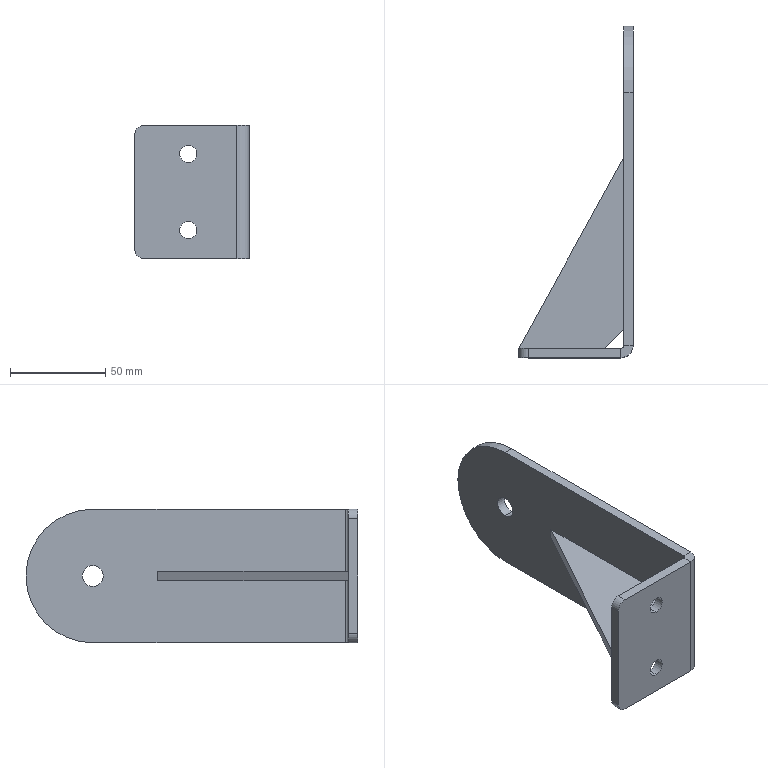Part | STEP file | 11-Unpowered roller support plate | 2 solids | 29 faces | box 60 x 174 x 70 mm | volume 89255 mm3 | plane 17 | cylinder 12 | commonest cylinder face diameters 9 x4 10 x2 11 x2 70 x2 3 x1 13 x1